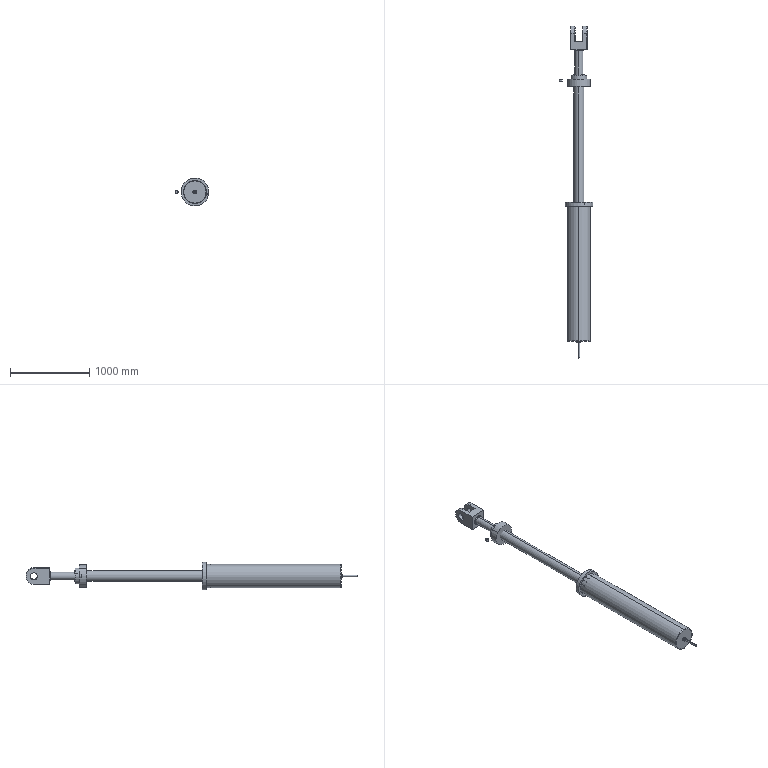Part | SolidWorks | features AEMSimFeature 1 | 13 solids | 442 faces | box 424.619 x 4179 x 350 mm | volume 96090471 mm3 | cylinder 220 | plane 128 | cone 88 | torus 6 | commonest cylinder face diameters 17.5 x32 21 x32 32 x32 220 x14 10 x10 14 x8